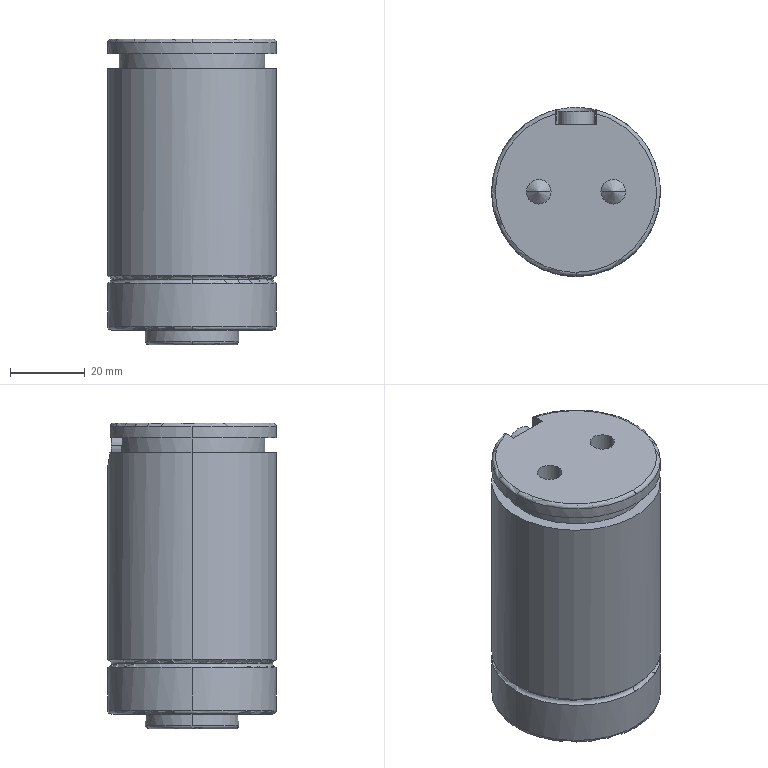Part | NX | features solid 2 | 1 solid | 55 faces | box 45.2 x 45.2 x 82 mm | volume 124227 mm3 | cylinder 21 | plane 16 | torus 10 | cone 8 | commonest cylinder face diameters 45.2 x7 6.6 x4 39.1 x3 4.9 x2 9.5 x2 25 x2